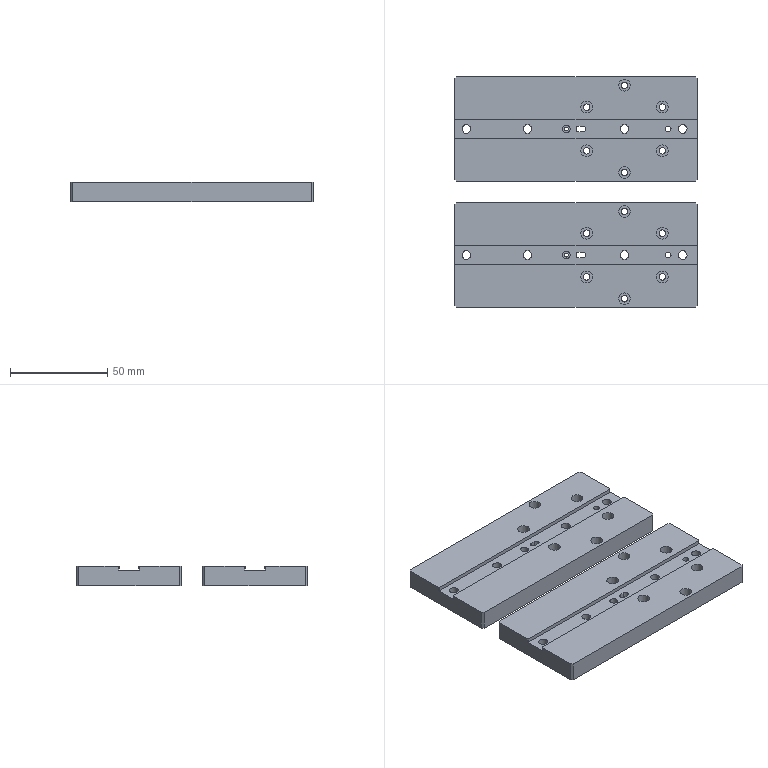NC program | NX | posted with a generic post | part box 125 x 119 x 10 mm
Whole program:
N10 G17 G21 G94 G90
(ZLEVEL_PROFILE_1_COPY_1_COPY_COPY_COPY , TOOL : D6A45)
N12 T22 M6
N14 G54
N16 G17 G0 G90 X-5.5 Y11.991 S7500 M3
N18 G43 Z30. H22
N20 Z1.
N22 G94 G1 Z-1. F1000.
N24 G3 X-6.241 Y11.25 R0.741
N26 X-5.5 Y11.991 R-0.741
N28 X-6.02 Y11.691 R0.6
N30 G1 Z0.
N32 G0 Z30.
N34 X-44.5 Y11.991
N36 Z1.
N38 G1 Z-1.
N40 G3 X-45.241 Y11.25 R0.741
N42 X-44.5 Y11.991 R-0.741
N44 X-45.02 Y11.691 R0.6
N46 G1 Z0.
N48 G0 Z30.
N50 X-3.5 Y-0.541
N52 Z1.
N54 G1 Z-1.
N56 X-1.5
N58 G3 X-0.959 Y0. R0.541
N60 X-1.5 Y0.541 R0.541
N62 G1 X-3.5
N64 G3 X-4.041 Y0. R0.541
N66 X-3.5 Y-0.541 R0.541
N68 X-2.98 Y-0.241 R0.6
N70 G1 Z0.
N72 G0 Z30.
N74 X-48.041 Y0.
N76 Z1.
N78 G1 Z-1.
N80 G3 X-47.5 Y-0.541 R0.541
N82 X-48.041 Y0. R-0.541
N84 X-47.891 Y-0.26 R0.3
N86 G1 Z0.
N88 G0 Z30.
N90 X57.649 Y-1.439
N92 Z0.
N94 G1 Z-1.
N96 X59.241 Y-0.52
N98 G3 X59.541 Y0. R0.6
N100 X56.5 Y3.041 R3.041
N102 X59.541 Y0. R-3.041
N104 X59.241 Y0.52 R0.6
N106 G1 X57.649 Y1.439
N108 Z0.
N110 G0 Z30.
N112 X-56.149
N114 Z0.
N116 G1 Z-1.
N118 X-57.741 Y0.52
N120 G3 X-58.041 Y0. R0.6
N122 X-55. Y-3.041 R3.041
N124 X-58.041 Y0. R-3.041
N126 X-57.741 Y-0.52 R0.6
N128 G1 X-56.149 Y-1.439
N130 Z0.
N132 G0 Z30.
N134 X23.561 Y-1.149
N136 Z0.
N138 G1 Z-1.
N140 X24.48 Y-2.741
N142 G3 X25. Y-3.041 R0.6
N144 X28.041 Y0. R3.041
N146 X25. Y-3.041 R-3.041
N148 X25.52 Y-2.741 R0.6
N150 G1 X26.439 Y-1.149
N152 Z0.
N154 G0 Z30.
N156 X-26.439
N158 Z0.
N160 G1 Z-1.
N162 X-25.52 Y-2.741
N164 G3 X-25. Y-3.041 R0.6
N166 X-21.959 Y0. R3.041
N168 X-25. Y-3.041 R-3.041
N170 X-24.48 Y-2.741 R0.6
N172 G1 X-23.561 Y-1.149
N174 Z0.
N176 G0 Z30.
N178 X-5.5 Y-11.991
N180 Z1.
N182 G1 Z-1.
N184 G3 X-4.759 Y-11.25 R0.741
N186 X-5.5 Y-11.991 R-0.741
N188 X-4.98 Y-11.691 R0.6
N190 G1 Z0.
N192 G0 Z30.
N194 X-44.5 Y-11.991
N196 Z1.
N198 G1 Z-1.
N200 G3 X-43.759 Y-11.25 R0.741
N202 X-44.5 Y-11.991 R-0.741
N204 X-43.98 Y-11.691 R0.6
N206 G1 Z0.
N208 G0 Z30.
N210 X-25. Y-23.241
N212 Z1.
N214 G1 Z-1.
N216 G3 X-24.259 Y-22.5 R0.741
N218 X-25. Y-23.241 R-0.741
N220 X-24.48 Y-22.941 R0.6
N222 G1 Z0.
N224 G0 Z30.
N226 X-25. Y23.241
N228 Z1.
N230 G1 Z-1.
N232 G3 X-25.741 Y22.5 R0.741
N234 X-25. Y23.241 R-0.741
N236 X-25.52 Y22.941 R0.6
N238 G1 Z0.
N240 G0 Z30.
N242 X-62.42 Y28.95
N244 Z0.
N246 G1 Z-1.
N248 X-62.02 Y28.259
N250 G3 X-61.501 Y27.959 R0.6
N252 G1 X61.501
N254 G2 X62.177 Y27.678 R0.992
N256 G1 X63.178 Y26.677
N258 G2 X63.459 Y26.001 R0.957
N260 G1 Y-26.001
N262 G2 X63.178 Y-26.677 R0.957
N264 G1 X62.177 Y-27.678
N266 G2 X61.501 Y-27.959 R0.992
N268 G1 X-61.501
N270 G2 X-62.177 Y-27.678 R0.992
N272 G1 X-63.178 Y-26.677
N274 G2 X-63.459 Y-26.001 R0.957
N276 G1 Y26.001
N278 G2 X-63.178 Y26.677 R0.957
N280 G1 X-62.177 Y27.678
N282 G2 X-61.501 Y27.959 R0.992
N284 G3 X-60.986 Y28.266 R0.6
N286 G1 X-60.488 Y29.159
N288 Z0.
N290 G0 Z30.
N292 M5
N294 M2